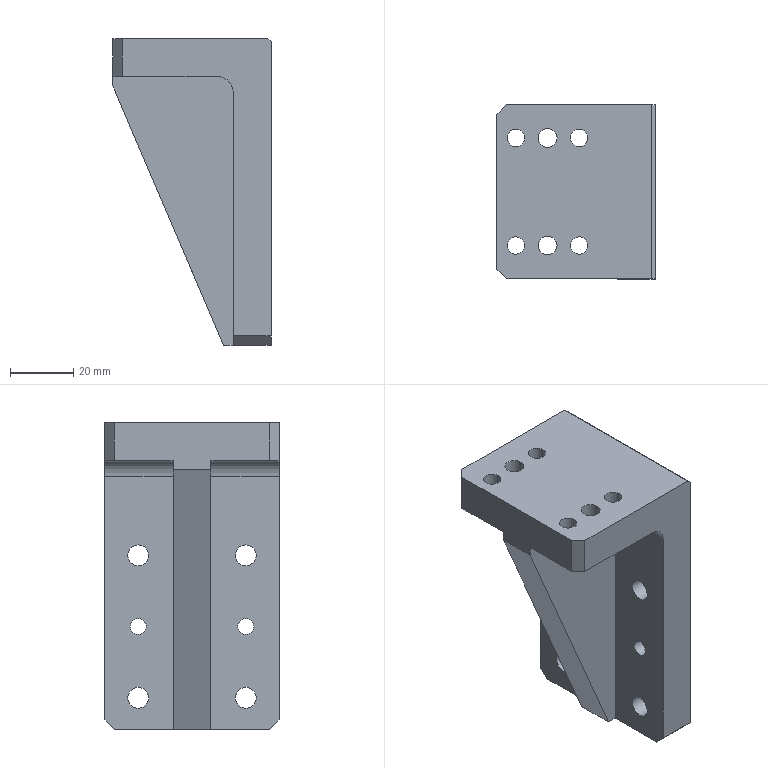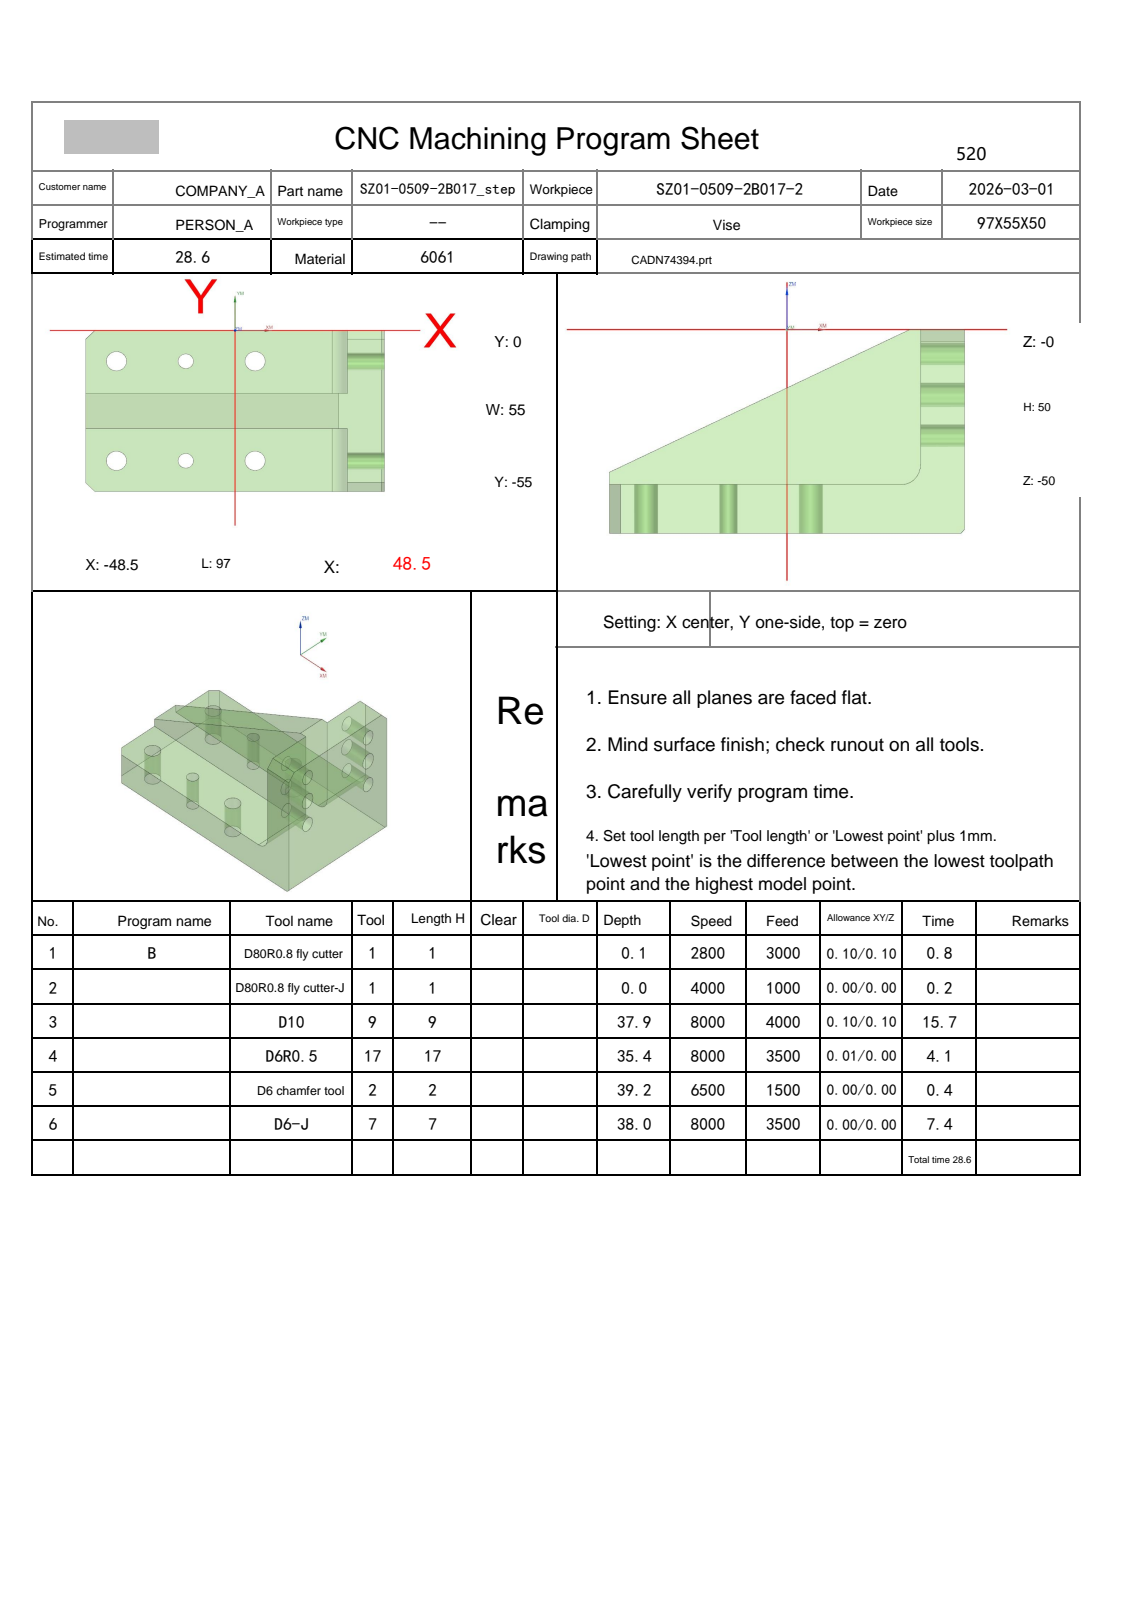NC program | NX | posted by the shop | part box 50 x 55 x 97 mm
Lines 8313 to 10086 of 18128:
N4 T17 M06
(D6R0.5  D=6. R=0.5 H=17 ce=0.01 di=0.00)
G00 G90 G54 X30.202 Y-.343 M03 S8000
G43 H17 Z14.5
M08
Z.429
G01 Z-.071 F3500.
X35.426 Y-.215
X35.55 Y-.212
X49.574
Y-.177 Z-.106
Y-.142 Z-.141
X35.55 Y-.141
X35.426 Y-.144
Y-.106 Z-.177
Y-.074 Z-.212
X35.55 Y-.071
X48.5
X49.574
Y-.035 Z-.247
X49.575 Y0.0 Z-.283
X48.5
X35.55
X35.425 Y-.003
Y.035 Z-.318
Y.068 Z-.354
X35.55 Y.071
X48.5
X49.575
Y.106 Z-.389
Y.141 Z-.424
X48.5
X35.55
X35.425 Y.138
X35.424 Y.177 Z-.46
Y.209 Z-.495
X35.55 Y.212
X48.5
X49.576
Y.247 Z-.53
Y.283 Z-.566
X48.5
X35.55
X35.424 Y.28
Y.318 Z-.601
X35.423 Y.35 Z-.636
X35.55 Y.354
X48.5
X49.577 Y.353
Y.389 Z-.672
Y.424 Z-.707
X48.5
X35.55
X35.423 Y.421
Y.46 Z-.742
Y.492 Z-.778
X35.55 Y.495
X48.5
X49.577
X49.578 Y.53 Z-.813
Y.566 Z-.849
X48.5
X35.55
X35.422 Y.563
Y.601 Z-.884
Y.633 Z-.919
X35.55 Y.636
X48.5
X49.578
Y.672 Z-.955
Y.707 Z-.99
X48.5
X35.55
X35.422 Y.704
X35.421 Y.742 Z-1.025
Y.775 Z-1.061
X35.55 Y.778
X48.5
X49.579
Y.813 Z-1.096
Y.848 Z-1.131
X48.5
X35.55
X35.421 Y.845
Y.884 Z-1.167
Y.916 Z-1.202
X35.55 Y.919
X48.5
X49.579
Y.955 Z-1.237
Y.99 Z-1.273
X48.5
X35.55
X35.421 Y.987
Y1.025 Z-1.308
Y1.058 Z-1.344
X35.55 Y1.061
X48.5
X49.579 Y1.06
Y1.096 Z-1.379
Y1.131 Z-1.414
X48.5
X36.5
X35.421
Y1.167 Z-1.45
Y1.199 Z-1.485
X35.55 Y1.202
X48.5
X49.579
Y1.237 Z-1.52
Y1.273 Z-1.556
X48.5
X35.55
X35.421 Y1.27
Y1.308 Z-1.591
Y1.34 Z-1.626
X35.55 Y1.343
X48.5
X49.579
Y1.379 Z-1.662
Y1.414 Z-1.697
X48.5
X35.55
X35.421 Y1.411
Y1.45 Z-1.732
Y1.482 Z-1.768
X35.55 Y1.485
X48.5
X49.579
Y1.52 Z-1.803
Y1.555 Z-1.838
X48.5 Y1.556
X35.55
X35.421 Y1.553
Y1.591 Z-1.874
Y1.623 Z-1.909
X35.55 Y1.626
X48.5
X49.579
Y1.662 Z-1.945
Y1.697 Z-1.98
X48.5
X35.55
X35.421 Y1.694
Y1.732 Z-2.015
Y1.765 Z-2.051
X35.55 Y1.768
X48.5
X49.579
Y1.803 Z-2.086
Y1.838 Z-2.121
X48.5
X35.55
X35.421 Y1.835
Y1.874 Z-2.157
Y1.906 Z-2.192
X35.55 Y1.909
X48.5
X49.579
Y1.944 Z-2.227
Y1.98 Z-2.263
X48.5
X35.55
X35.421 Y1.977
X35.422 Y2.015 Z-2.298
Y2.048 Z-2.333
X35.55 Y2.051
X48.5
X49.578 Y2.05
Y2.086 Z-2.369
Y2.121 Z-2.404
X48.5
X35.55
X35.422 Y2.118
Y2.157 Z-2.44
Y2.189 Z-2.475
X35.55 Y2.192
X48.5
X49.578
X49.577 Y2.227 Z-2.51
Y2.263 Z-2.546
X48.5
X35.55
X35.423 Y2.26
Y2.298 Z-2.581
Y2.33 Z-2.616
X35.55 Y2.333
X48.5
X49.577
Y2.369 Z-2.652
X49.576 Y2.404 Z-2.687
X48.5
X35.55
X35.424 Y2.401
Y2.439 Z-2.722
Y2.472 Z-2.758
X35.55 Y2.475
X48.5
X49.576
Y2.505 Z-2.788
Y2.535 Z-2.818
X48.5
X35.55
X35.424 Y2.532
X35.425 Y2.566 Z-2.849
Y2.593 Z-2.879
X35.55 Y2.596
X48.5
X49.575
Y2.626 Z-2.909
Y2.656 Z-2.939
X48.5 Y2.657
X35.55
X35.425 Y2.654
Y2.687 Z-2.97
Y2.714 Z-3.
X35.55 Y2.717
X48.5
X49.575
G00 Z14.5
X54.722 Y-54.788
Z.429
G01 Z-.071
X49.574
X35.552
X35.427 Y-54.785
X35.426 Y-54.823 Z-.106
Y-54.856 Z-.141
X35.552 Y-54.859
X49.574 Y-54.858
Y-54.894 Z-.177
Y-54.929 Z-.212
X48.5
X35.552
X35.426 Y-54.926
X35.425 Y-54.965 Z-.247
Y-54.997 Z-.283
X35.552 Y-55.
X48.5
X49.575
Y-55.035 Z-.318
Y-55.071 Z-.354
X48.5
X35.552
X35.425 Y-55.068
Y-55.106 Z-.389
Y-55.138 Z-.424
X35.552 Y-55.141
X48.5
X49.575
X49.576 Y-55.177 Z-.46
Y-55.212 Z-.495
X48.5
X35.552
X35.424 Y-55.209
Y-55.247 Z-.53
Y-55.28 Z-.566
X35.552 Y-55.283
X48.5
X49.576
Y-55.318 Z-.601
X49.577 Y-55.353 Z-.636
X48.5 Y-55.354
X35.552
X35.423 Y-55.35
Y-55.389 Z-.672
Y-55.421 Z-.707
X35.552 Y-55.424
X48.5
X49.577
Y-55.46 Z-.742
Y-55.495 Z-.778
X48.5
X35.552
X35.423 Y-55.492
Y-55.53 Z-.813
X35.422 Y-55.563 Z-.849
X35.552 Y-55.566
X48.5
X49.578 Y-55.565
Y-55.601 Z-.884
Y-55.636 Z-.919
X48.5
X35.552
X35.422 Y-55.633
Y-55.672 Z-.955
Y-55.704 Z-.99
X35.552 Y-55.707
X48.5
X49.579
Y-55.742 Z-1.025
Y-55.778 Z-1.061
X48.5
X35.552
X35.421 Y-55.775
Y-55.813 Z-1.096
Y-55.845 Z-1.131
X35.552 Y-55.848
X48.5
X49.579
Y-55.884 Z-1.167
Y-55.919 Z-1.202
X48.5
X35.552
X35.421 Y-55.916
Y-55.955 Z-1.237
Y-55.987 Z-1.273
X35.552 Y-55.99
X48.5
X49.579
Y-56.025 Z-1.308
Y-56.06 Z-1.344
X48.5 Y-56.061
X35.552
X35.421 Y-56.058
Y-56.096 Z-1.379
Y-56.131 Z-1.414
X36.5
X48.5
X49.579
Y-56.167 Z-1.45
Y-56.202 Z-1.485
X48.5
X35.552
X35.421 Y-56.199
Y-56.237 Z-1.52
Y-56.27 Z-1.556
X35.552 Y-56.273
X48.5
X49.579
Y-56.308 Z-1.591
Y-56.343 Z-1.626
X48.5
X35.552
X35.421 Y-56.34
Y-56.379 Z-1.662
Y-56.411 Z-1.697
X35.552 Y-56.414
X48.5
X49.579
Y-56.45 Z-1.732
Y-56.485 Z-1.768
X48.5
X35.552
X35.421 Y-56.482
Y-56.52 Z-1.803
Y-56.553 Z-1.838
X35.552 Y-56.556
X48.5
X49.579 Y-56.555
Y-56.591 Z-1.874
Y-56.626 Z-1.909
X48.5
X35.552
X35.421 Y-56.623
Y-56.662 Z-1.945
Y-56.694 Z-1.98
X35.552 Y-56.697
X48.5
X49.579
Y-56.732 Z-2.015
Y-56.768 Z-2.051
X48.5
X35.552
X35.421 Y-56.765
Y-56.803 Z-2.086
Y-56.835 Z-2.121
X35.552 Y-56.838
X48.5
X49.579
Y-56.874 Z-2.157
Y-56.909 Z-2.192
X48.5
X35.552
X35.421 Y-56.906
Y-56.944 Z-2.227
Y-56.977 Z-2.263
X35.552 Y-56.98
X48.5
X49.579
X49.578 Y-57.015 Z-2.298
Y-57.05 Z-2.333
X48.5 Y-57.051
X35.552
X35.422 Y-57.048
Y-57.086 Z-2.369
Y-57.118 Z-2.404
X35.552 Y-57.121
X48.5
X49.578
Y-57.157 Z-2.44
X49.577 Y-57.192 Z-2.475
X48.5
X35.552
X35.422 Y-57.189
X35.423 Y-57.227 Z-2.51
Y-57.26 Z-2.546
X35.552 Y-57.263
X48.5
X49.577
Y-57.298 Z-2.581
Y-57.333 Z-2.616
X48.5
X35.552
X35.423 Y-57.33
Y-57.369 Z-2.652
X35.424 Y-57.401 Z-2.687
X35.552 Y-57.404
X48.5
X49.576
Y-57.439 Z-2.722
Y-57.475 Z-2.758
X48.5
X35.552
X35.424 Y-57.472
Y-57.505 Z-2.788
Y-57.532 Z-2.818
X35.552 Y-57.535
X48.5
X49.576
Y-57.566 Z-2.849
X49.575 Y-57.596 Z-2.879
X48.5
X35.552
X35.425 Y-57.593
Y-57.626 Z-2.909
Y-57.654 Z-2.939
X35.552 Y-57.657
X48.5
X49.575 Y-57.656
Y-57.687 Z-2.97
Y-57.717 Z-3.
X48.5
X35.552
X35.425 Y-57.714
G00 Z14.5
G00 G90 X27.799 Y-34.576 M03 S8000
Z14.5
Z.461
G01 Z-.039 F3500.
X30.799
Y-20.424
X30.75 Z-.059
X30.707 Z-.079
X30.704 Y-21.5
Y-33.5
X30.707 Y-34.576
X30.658 Y-34.577 Z-.098
X30.615 Z-.118
X30.612 Y-33.5
Y-21.5
X30.615 Y-20.423
X30.566 Z-.137
X30.523 Z-.157
X30.52 Y-21.5
Y-33.5
X30.523 Y-34.577
X30.474 Y-34.578 Z-.177
X30.431 Z-.196
X30.428 Y-33.5
Y-21.5
X30.431 Y-20.422
X30.382 Z-.216
X30.339 Y-20.421 Z-.236
X30.336 Y-21.5
Y-33.5
X30.339 Y-34.578
X30.29 Y-34.579 Z-.255
X30.247 Z-.275
X30.244 Y-33.5
Y-21.5
X30.247 Y-20.421
X30.198 Z-.294
X30.155 Y-20.42 Z-.314
X30.152 Y-21.5
Y-33.5
X30.155 Y-34.58
X30.106 Z-.334
X30.063 Z-.353
X30.06 Y-33.5
Y-21.5
X30.063 Y-20.42
X30.014 Y-20.419 Z-.373
X29.971 Z-.393
X29.968 Y-21.5
Y-33.5
X29.971 Y-34.581
X29.922 Z-.412
X29.879 Z-.432
X29.876 Y-33.5
Y-21.5
X29.879 Y-20.419
X29.83 Y-20.418 Z-.451
X29.787 Z-.471
X29.784 Y-21.5
Y-33.5
X29.787 Y-34.582
X29.738 Z-.491
X29.695 Y-34.583 Z-.51
X29.692 Y-33.5
Y-21.5
X29.695 Y-20.418
X29.646 Y-20.417 Z-.53
X29.603 Z-.55
X29.6 Y-21.5
Y-33.5
X29.603 Y-34.583
X29.554 Z-.569
X29.511 Y-34.584 Z-.589
X29.508 Y-33.5
Y-21.5
X29.511 Y-20.416
X29.462 Z-.608
X29.419 Z-.628
X29.416 Y-21.5
Y-33.5
X29.419 Y-34.584
X29.37 Y-34.585 Z-.648
X29.327 Z-.667
X29.324 Y-33.5
Y-21.5
X29.327 Y-20.415
X29.278 Z-.687
X29.235 Z-.707
X29.232 Y-21.5
Y-33.5
X29.235 Y-34.585
X29.186 Y-34.586 Z-.726
X29.143 Z-.746
X29.14 Y-33.5
Y-21.5
X29.143 Y-20.414
X29.094 Z-.766
X29.051 Z-.785
X29.048 Y-21.5
Y-33.5
X29.051 Y-34.586
X29.002 Y-34.587 Z-.805
X28.959 Z-.824
X28.956 Y-33.5
Y-21.5
X28.959 Y-20.413
X28.91 Z-.844
X28.867 Z-.864
X28.864 Y-21.5
Y-33.5
X28.867 Y-34.587
X28.818 Y-34.588 Z-.883
X28.775 Z-.903
X28.772 Y-33.5
Y-21.5
X28.775 Y-20.412
X28.726 Z-.923
X28.683 Z-.942
X28.68 Y-21.5
Y-33.5
X28.683 Y-34.588
X28.634 Z-.962
X28.591 Y-34.589 Z-.981
X28.588 Y-33.5
Y-21.5
X28.591 Y-20.411
X28.542 Z-1.001
X28.499 Z-1.021
X28.496 Y-21.5
Y-33.5
X28.499 Y-34.589
X28.45 Z-1.04
X28.407 Y-34.59 Z-1.06
X28.405 Y-33.5
Y-21.5
X28.407 Y-20.411
X28.359 Y-20.41 Z-1.08
X28.315 Z-1.099
X28.313 Y-21.5
Y-33.5
X28.315 Y-34.59
X28.267 Z-1.119
X28.223 Z-1.138
X28.221 Y-33.5
Y-21.5
X28.223 Y-20.41
X28.175 Z-1.158
X28.131 Y-20.409 Z-1.178
X28.129 Y-21.5
Y-33.5
X28.131 Y-34.591
X28.083 Z-1.197
X28.039 Z-1.217
X28.037 Y-33.5
Y-21.5
X28.039 Y-20.409
X27.991 Z-1.237
X27.947 Z-1.256
X27.945 Y-21.5
Y-33.5
X27.947 Y-34.591
X27.899 Y-34.592 Z-1.276
X27.855 Z-1.295
X27.853 Y-33.5
Y-21.5
X27.855 Y-20.408
X27.807 Z-1.315
X27.763 Z-1.335
X27.761 Y-21.5
Y-33.5
X27.763 Y-34.592
X27.715 Z-1.354
X27.671 Y-34.593 Z-1.374
X27.669 Y-33.5
Y-21.5
X27.671 Y-20.407
X27.623 Z-1.394
X27.579 Z-1.413
X27.577 Y-21.5
Y-33.5
X27.579 Y-34.593
X27.531 Z-1.433
X27.487 Z-1.452
X27.485 Y-33.5
Y-21.5
X27.487 Y-20.407
X27.439 Y-20.406 Z-1.472
X27.395 Z-1.492
X27.393 Y-21.5
Y-33.5
X27.395 Y-34.594
X27.347 Z-1.511
X27.303 Z-1.531
X27.301 Y-33.5
Y-21.5
X27.303 Y-20.406
X27.255 Z-1.551
X27.211 Z-1.57
X27.209 Y-21.5
Y-33.5
X27.211 Y-34.594
X27.163 Y-34.595 Z-1.59
X27.119 Z-1.61
X27.117 Y-33.5
Y-21.5
X27.119 Y-20.405
X27.071 Z-1.629
X27.027 Z-1.649
X27.025 Y-21.5
Y-33.5
X27.027 Y-34.595
X26.979 Z-1.668
X26.935 Z-1.688
X26.933 Y-33.5
Y-21.5
X26.935 Y-20.405
X26.887 Z-1.708
X26.843 Z-1.727
X26.841 Y-21.5
Y-33.5
X26.843 Y-34.595
X26.795 Y-34.596 Z-1.747
X26.751 Z-1.767
X26.749 Y-33.5
Y-21.5
X26.751 Y-20.404
X26.703 Z-1.786
X26.659 Z-1.806
X26.657 Y-21.5
Y-33.5
X26.659 Y-34.596
X26.611 Z-1.825
X26.567 Z-1.845
X26.565 Y-33.5
Y-21.5
X26.567 Y-20.404
X26.519 Z-1.865
X26.475 Z-1.884
X26.473 Y-21.5
Y-33.5
X26.475 Y-34.596
X26.427 Z-1.904
X26.383 Z-1.924
X26.381 Y-33.5
Y-21.5
X26.383 Y-20.404
X26.335 Z-1.943
X26.292 Y-20.403 Z-1.963
X26.289 Y-21.5
Y-33.5
X26.292 Y-34.597
X26.243 Z-1.982
X26.2 Z-2.002
X26.197 Y-33.5
Y-21.5
X26.2 Y-20.403
X26.151 Z-2.022
X26.108 Z-2.041
X26.105 Y-21.5
Y-33.5
X26.108 Y-34.597
X26.059 Z-2.061
X26.016 Z-2.081
X26.013 Y-33.5
Y-21.5
X26.016 Y-20.403
X25.967 Z-2.1
X25.924 Z-2.12
X25.921 Y-21.5
Y-33.5
X25.924 Y-34.597
X25.875 Z-2.139
X25.832 Z-2.159
X25.829 Y-33.5
Y-21.5
X25.832 Y-20.403
X25.783 Z-2.179
X25.74 Y-20.402 Z-2.198
X25.737 Y-21.5
Y-33.5
X25.74 Y-34.598
X25.691 Z-2.218
X25.648 Z-2.238
X25.645 Y-33.5
Y-21.5
X25.648 Y-20.402
X25.599 Z-2.257
X25.556 Z-2.277
X25.553 Y-21.5
Y-33.5
X25.556 Y-34.598
X25.507 Z-2.297
X25.464 Z-2.316
X25.461 Y-33.5
Y-21.5
X25.464 Y-20.402
X25.415 Z-2.336
X25.372 Z-2.355
X25.369 Y-21.5
Y-33.5
X25.372 Y-34.598
X25.323 Z-2.375
X25.28 Z-2.395
X25.277 Y-33.5
Y-21.5
X25.28 Y-20.402
X25.231 Z-2.414
X25.188 Z-2.434
X25.185 Y-21.5
Y-33.5
X25.188 Y-34.598
X25.139 Z-2.454
X25.096 Z-2.473
X25.093 Y-33.5
Y-21.5
X25.096 Y-20.401
X25.048 Z-2.493
X25.004 Z-2.512
X25.002 Y-21.5
Y-33.5
X25.004 Y-34.598
X24.956 Z-2.532
X24.912 Y-34.599 Z-2.552
X24.91 Y-33.5
Y-21.5
X24.912 Y-20.401
X24.864 Z-2.571
X24.82 Z-2.591
X24.818 Y-21.5
Y-33.5
X24.82 Y-34.599
X24.772 Z-2.611
X24.728 Z-2.63
X24.726 Y-33.5
Y-21.5
X24.728 Y-20.401
X24.68 Z-2.65
X24.636 Z-2.669
X24.634 Y-21.5
Y-33.5
X24.636 Y-34.599
X24.588 Z-2.689
X24.544 Z-2.709
X24.542 Y-33.5
Y-21.5
X24.544 Y-20.401
X24.496 Z-2.728
X24.452 Z-2.748
X24.45 Y-21.5
Y-33.5
X24.452 Y-34.599
X24.404 Z-2.768
X24.36 Z-2.787
X24.358 Y-33.5
Y-21.5
X24.36 Y-20.401
X24.312 Z-2.807
X24.268 Z-2.826
X24.266 Y-21.5
Y-33.5
X24.268 Y-34.599
X24.22 Z-2.846
X24.176 Z-2.866
X24.174 Y-33.5
Y-21.5
X24.176 Y-20.401
X24.128 Z-2.885
X24.084 Z-2.905
X24.082 Y-21.5
Y-33.5
X24.084 Y-34.599
X24.036 Z-2.925
X23.992 Z-2.944
X23.99 Y-33.5
Y-21.5
X23.992 Y-20.401
X23.944 Z-2.964
X23.9 Z-2.983
X23.898 Y-21.5
Y-33.5
X23.9 Y-34.599
X23.852 Z-3.003
X23.808 Z-3.023
X23.806 Y-33.5
Y-21.5
X23.808 Y-20.401
X23.76 Z-3.042
X23.716 Z-3.062
X23.714 Y-21.5
Y-33.5
X23.716 Y-34.599
X23.668 Z-3.082
X23.624 Z-3.101
X23.622 Y-33.5
Y-21.5
X23.624 Y-20.401
X23.576 Z-3.121
X23.532 Z-3.141
X23.53 Y-21.5
Y-33.5
X23.532 Y-34.599
X23.484 Z-3.16
X23.44 Z-3.18
X23.438 Y-33.5
Y-21.5
X23.44 Y-20.401
X23.392 Z-3.199
X23.348 Y-20.4 Z-3.219
X23.346 Y-21.5
Y-33.5
X23.348 Y-34.599
X23.3 Z-3.239
X23.256 Z-3.258
X23.254 Y-33.5
Y-21.5
X23.256 Y-20.4
X23.208 Z-3.278
X23.164 Z-3.298
X23.162 Y-21.5
Y-33.5
X23.164 Y-34.599
X23.116 Y-34.6 Z-3.317
X23.072 Z-3.337
X23.07 Y-33.5
Y-21.5
X23.072 Y-20.4
X23.024 Z-3.356
X22.98 Z-3.376
X22.978 Y-21.5
Y-33.5
X22.98 Y-34.6
X22.932 Z-3.396
X22.888 Z-3.415
X22.886 Y-33.5
Y-21.5
X22.888 Y-20.4
X22.84 Z-3.435
X22.797 Z-3.455
X22.794 Y-21.5
Y-33.5
X22.797 Y-34.6
X22.748 Z-3.474
X22.705 Z-3.494
X22.702 Y-33.5
Y-21.5
X22.705 Y-20.4
X22.656 Z-3.513
X22.613 Z-3.533
X22.61 Y-21.5
Y-33.5
X22.613 Y-34.6
X22.564 Z-3.553
X22.521 Z-3.572
X22.518 Y-33.5
Y-21.5
X22.521 Y-20.4
X22.472 Z-3.592
X22.429 Z-3.612
X22.426 Y-21.5
Y-33.5
X22.429 Y-34.6
X22.38 Z-3.631
X22.337 Z-3.651
X22.334 Y-33.5
Y-21.5
X22.337 Y-20.4
X22.288 Z-3.67
X22.245 Z-3.69
X22.242 Y-21.5
Y-33.5
X22.245 Y-34.6
X22.196 Z-3.71
X22.153 Z-3.729
X22.15 Y-33.5
Y-21.5
X22.153 Y-20.4
X22.104 Z-3.749
X22.061 Z-3.769
X22.058 Y-21.5
Y-33.5
X22.061 Y-34.6
X22.012 Z-3.788
X21.969 Z-3.808
X21.966 Y-33.5
Y-21.5
X21.969 Y-20.4
X21.92 Z-3.828
X21.877 Z-3.847
X21.874 Y-21.5
Y-33.5
X21.877 Y-34.6
X21.828 Z-3.867
X21.785 Z-3.886
X21.782 Y-33.5
Y-21.5
X21.785 Y-20.4
X21.736 Z-3.906
X21.693 Z-3.926
X21.691 Y-21.5
Y-33.5
X21.693 Y-34.6
X21.645 Z-3.945
X21.601 Z-3.965
X21.599 Y-33.5
Y-21.5
X21.601 Y-20.4
X21.553 Z-3.985
X21.509 Z-4.004
X21.507 Y-21.5
Y-33.5
X21.509 Y-34.6
X21.461 Z-4.024
X21.417 Z-4.043
X21.415 Y-33.5
Y-21.5
X21.417 Y-20.4
X21.369 Z-4.063
X21.325 Z-4.083
X21.323 Y-21.5
Y-33.5
X21.325 Y-34.6
X21.277 Z-4.102
X21.233 Z-4.122
X21.231 Y-33.5
Y-21.5
X21.233 Y-20.4
X21.185 Z-4.142
X21.141 Z-4.161
X21.139 Y-21.5
Y-33.5
X21.141 Y-34.6
X21.093 Z-4.181
X21.049 Z-4.2
X21.047 Y-33.5
Y-21.5
X21.049 Y-20.4
X21.001 Z-4.22
X20.957 Z-4.24
X20.955 Y-21.5
Y-33.5
X20.957 Y-34.6
X20.909 Z-4.259
X20.865 Z-4.279
X20.863 Y-33.5
Y-21.5
X20.865 Y-20.4
X20.817 Z-4.299
X20.773 Z-4.318
X20.771 Y-21.5
Y-33.5
X20.773 Y-34.6
X20.725 Z-4.338
X20.681 Z-4.357
X20.679 Y-33.5
Y-21.5
X20.681 Y-20.4
X20.633 Z-4.377
X20.589 Z-4.397
X20.587 Y-21.5
Y-33.5
X20.589 Y-34.6
X20.541 Z-4.416
X20.497 Z-4.436
X20.495 Y-33.5
Y-21.5
X20.497 Y-20.4
X20.449 Z-4.456
X20.405 Z-4.475
X20.403 Y-21.5
Y-33.5
X20.405 Y-34.6
X20.357 Z-4.495
X20.313 Z-4.515
X20.311 Y-33.5
Y-21.5
X20.313 Y-20.4
X20.265 Z-4.534
X20.221 Z-4.554
X20.219 Y-21.5
Y-33.5
X20.221 Y-34.6
X20.173 Z-4.573
X20.129 Z-4.593
X20.127 Y-33.5
Y-21.5
X20.129 Y-20.4
X20.081 Z-4.613
X20.037 Z-4.632
X20.035 Y-21.5
Y-33.5
X20.037 Y-34.6
X19.989 Z-4.652
X19.945 Z-4.672
X19.943 Y-33.5
Y-21.5
X19.945 Y-20.4
X19.897 Z-4.691
X19.853 Z-4.711
X19.851 Y-21.5
Y-33.5
X19.853 Y-34.6
X19.805 Z-4.73
X19.761 Z-4.75
X19.759 Y-33.5
Y-21.5
X19.761 Y-20.4
X19.713 Z-4.77
X19.669 Z-4.789
X19.667 Y-21.5
Y-33.5
X19.669 Y-34.6
X19.621 Z-4.809
X19.577 Z-4.829
X19.575 Y-33.5
Y-21.5
X19.577 Y-20.4
X19.529 Z-4.848
X19.485 Z-4.868
X19.483 Y-21.5
Y-33.5
X19.485 Y-34.6
X19.437 Z-4.887
X19.394 Z-4.907
X19.391 Y-33.5
Y-21.5
X19.394 Y-20.4
X19.345 Z-4.927
X19.302 Z-4.946
X19.299 Y-21.5
Y-33.5
X19.302 Y-34.6
X19.253 Z-4.966
X19.21 Z-4.986
X19.207 Y-33.5
Y-21.5
X19.21 Y-20.4
X19.161 Z-5.005
X19.118 Z-5.025
X19.115 Y-21.5
Y-33.5
X19.118 Y-34.6
X19.069 Z-5.044
X19.026 Z-5.064
X19.023 Y-33.5
Y-21.5
X19.026 Y-20.4
X18.977 Z-5.084
X18.934 Z-5.103
X18.931 Y-21.5
Y-33.5
X18.934 Y-34.6
X18.885 Z-5.123
X18.842 Z-5.143
X18.839 Y-33.5
Y-21.5
X18.842 Y-20.4
X18.793 Z-5.162
X18.75 Z-5.182
X18.747 Y-21.5
Y-33.5
X18.75 Y-34.6
X18.701 Z-5.201
X18.658 Z-5.221
X18.655 Y-33.5
Y-21.5
X18.658 Y-20.4
X18.609 Z-5.241
X18.566 Z-5.26
X18.563 Y-21.5
Y-33.5
X18.566 Y-34.6
X18.517 Z-5.28
X18.474 Z-5.3
X18.471 Y-33.5
Y-21.5
X18.474 Y-20.4
X18.425 Z-5.319
X18.382 Z-5.339
X18.38 Y-21.5
Y-33.5
X18.382 Y-34.6
X18.334 Z-5.359
X18.29 Z-5.378
X18.288 Y-33.5
Y-21.5
X18.29 Y-20.4
X18.242 Z-5.398
X18.198 Z-5.417
X18.196 Y-21.5
Y-33.5
X18.198 Y-34.6
X18.15 Z-5.437
X18.106 Z-5.457
X18.104 Y-33.5
Y-21.5
X18.106 Y-20.4
X18.058 Z-5.476
X18.014 Z-5.496
X18.012 Y-21.5
Y-33.5
X18.014 Y-34.6
X17.966 Z-5.516
X17.922 Z-5.535
X17.92 Y-33.5
Y-21.5
X17.922 Y-20.4
X17.874 Z-5.555
X17.83 Z-5.574
X17.828 Y-21.5
Y-33.5
X17.83 Y-34.6
X17.782 Z-5.594
X17.738 Z-5.614
X17.736 Y-33.5
Y-21.5
X17.738 Y-20.4
X17.69 Z-5.633
X17.646 Z-5.653
X17.644 Y-21.5
Y-33.5
X17.646 Y-34.6
X17.598 Z-5.673
X17.554 Z-5.692
X17.552 Y-33.5
Y-21.5
X17.554 Y-20.4
X17.506 Z-5.712
X17.462 Z-5.731
X17.46 Y-21.5
Y-33.5
X17.462 Y-34.6
X17.414 Z-5.751
X17.37 Z-5.771
X17.368 Y-33.5
Y-21.5
X17.37 Y-20.4
X17.322 Z-5.79
X17.278 Z-5.81
X17.276 Y-21.5
Y-33.5
X17.278 Y-34.6
X17.23 Z-5.83
X17.186 Z-5.849
X17.184 Y-33.5
Y-21.5
X17.186 Y-20.4
X17.138 Z-5.869
X17.094 Z-5.888
X17.092 Y-21.5
Y-33.5
X17.094 Y-34.6
X17.046 Z-5.908
X17.002 Z-5.928
X17. Y-33.5
Y-21.5
X17.002 Y-20.4
X16.954 Z-5.947
X16.91 Z-5.967
X16.908 Y-21.5
Y-33.5
X16.91 Y-34.6
X16.862 Z-5.987
X16.818 Z-6.006
X16.816 Y-33.5
Y-21.5
X16.818 Y-20.4
X16.77 Z-6.026
X16.726 Z-6.046
X16.724 Y-21.5
Y-33.5
X16.726 Y-34.6
X16.678 Z-6.065
X16.634 Z-6.085
X16.632 Y-33.5
Y-21.5
X16.634 Y-20.4
X16.586 Z-6.104
X16.542 Z-6.124
X16.54 Y-21.5
Y-33.5
X16.542 Y-34.6
X16.494 Z-6.144
X16.45 Z-6.163
X16.448 Y-33.5
Y-21.5
X16.45 Y-20.4
X16.402 Z-6.183
X16.358 Z-6.203
X16.356 Y-21.5
Y-33.5
X16.358 Y-34.6
X16.31 Z-6.222
X16.266 Z-6.242
X16.264 Y-33.5
Y-21.5
X16.266 Y-20.4
X16.218 Z-6.261
X16.174 Z-6.281
X16.172 Y-21.5
Y-33.5
X16.174 Y-34.6
X16.126 Z-6.301
X16.083 Z-6.32
X16.08 Y-33.5
Y-21.5
X16.083 Y-20.4
X16.034 Z-6.34
X15.99 Z-6.36
X15.988 Y-21.5
Y-33.5
X15.99 Y-34.6
X15.942 Z-6.379
X15.899 Z-6.399
X15.896 Y-33.5
Y-21.5
X15.899 Y-20.4
X15.85 Z-6.418
X15.807 Z-6.438
X15.804 Y-21.5
Y-33.5
X15.807 Y-34.6
X15.758 Z-6.458
X15.715 Z-6.477
X15.712 Y-33.5
Y-21.5
X15.715 Y-20.4
X15.666 Z-6.497
X15.623 Z-6.517
X15.62 Y-21.5
Y-33.5
X15.623 Y-34.6
X15.574 Z-6.536
X15.531 Z-6.556
X15.528 Y-33.5
Y-21.5
X15.531 Y-20.4
X15.482 Z-6.575
X15.439 Z-6.595
X15.436 Y-21.5
Y-33.5
X15.439 Y-34.6
X15.39 Z-6.615
X15.347 Z-6.634
X15.344 Y-33.5
Y-21.5
X15.347 Y-20.4
X15.298 Z-6.654
X15.255 Z-6.674
X15.252 Y-21.5
Y-33.5
X15.255 Y-34.6
X15.206 Z-6.693
X15.163 Z-6.713
X15.16 Y-33.5
Y-21.5
X15.163 Y-20.4
X15.114 Z-6.732
X15.071 Z-6.752
X15.068 Y-21.5
Y-33.5
X15.071 Y-34.6
X15.023 Z-6.772
X14.979 Z-6.791
X14.977 Y-33.5
Y-21.5
X14.979 Y-20.4
X14.931 Z-6.811
X14.887 Z-6.831
X14.885 Y-21.5
Y-33.5
X14.887 Y-34.6
X14.839 Z-6.85
X14.795 Z-6.87
X14.793 Y-33.5
Y-21.5
X14.795 Y-20.4
X14.747 Z-6.89
X14.703 Z-6.909
X14.701 Y-21.5
Y-33.5
X14.703 Y-34.6
X14.655 Z-6.929
X14.611 Z-6.948
X14.609 Y-33.5
Y-21.5
X14.611 Y-20.4
X14.563 Z-6.968
X14.519 Z-6.988
X14.517 Y-21.5
Y-33.5
X14.519 Y-34.6
X14.471 Z-7.007
X14.427 Z-7.027
X14.425 Y-33.5
Y-21.5
X14.427 Y-20.4
X14.379 Z-7.047
X14.335 Z-7.066
X14.333 Y-21.5
Y-33.5
X14.335 Y-34.6
X14.287 Z-7.086
X14.243 Z-7.105
X14.241 Y-33.5
Y-21.5
X14.243 Y-20.4
X14.195 Z-7.125
X14.151 Z-7.145
X14.149 Y-21.5
Y-33.5
X14.151 Y-34.6
X14.103 Z-7.164
X14.059 Z-7.184
X14.057 Y-33.5
Y-21.5
X14.059 Y-20.4
X14.011 Z-7.204
X13.967 Z-7.223
X13.965 Y-21.5
Y-33.5
X13.967 Y-34.6
X13.919 Z-7.243
X13.875 Z-7.262
X13.873 Y-33.5
Y-21.5
X13.875 Y-20.4
X13.827 Z-7.282
X13.783 Z-7.302
X13.781 Y-21.5
Y-33.5
X13.783 Y-34.6
X13.735 Z-7.321
X13.691 Z-7.341
X13.689 Y-33.5
Y-21.5
X13.691 Y-20.4
X13.643 Z-7.361
X13.599 Z-7.38
X13.597 Y-21.5
Y-33.5
X13.599 Y-34.6
X13.551 Z-7.4
X13.507 Z-7.419
X13.505 Y-33.5
Y-21.5
X13.507 Y-20.4
X13.459 Z-7.439
X13.415 Z-7.459
X13.413 Y-21.5
Y-33.5
X13.415 Y-34.6
X13.367 Z-7.478
X13.323 Z-7.498
X13.321 Y-33.5
Y-21.5
X13.323 Y-20.4
X13.275 Z-7.518
X13.231 Z-7.537
X13.229 Y-21.5
Y-33.5
X13.231 Y-34.6
X13.183 Z-7.557
X13.139 Z-7.577
X13.137 Y-33.5
Y-21.5
X13.139 Y-20.4
X13.091 Z-7.596
X13.047 Z-7.616
X13.045 Y-21.5
Y-33.5
X13.047 Y-34.6
X12.999 Z-7.635
X12.955 Z-7.655
X12.953 Y-33.5
Y-21.5
X12.955 Y-20.4
X12.907 Z-7.675
X12.863 Z-7.694
X12.861 Y-21.5
Y-33.5
X12.863 Y-34.6
X12.815 Z-7.714
X12.772 Z-7.734
X12.769 Y-33.5
Y-21.5
X12.772 Y-20.4
X12.723 Z-7.753
X12.68 Z-7.773
X12.677 Y-21.5
Y-33.5
X12.68 Y-34.6
X12.631 Z-7.792
X12.588 Z-7.812
X12.585 Y-33.5
Y-21.5
X12.588 Y-20.4
X12.539 Z-7.832
X12.496 Z-7.851
X12.493 Y-21.5
Y-33.5
X12.496 Y-34.6
X12.447 Z-7.871
X12.404 Z-7.891
X12.401 Y-33.5
Y-21.5
X12.404 Y-20.4
X12.355 Z-7.91
X12.312 Z-7.93
X12.309 Y-21.5
Y-33.5
X12.312 Y-34.6
X12.263 Z-7.949
X12.22 Z-7.969
X12.217 Y-33.5
Y-21.5
X12.22 Y-20.4
X12.171 Z-7.989
X12.128 Z-8.008
X12.125 Y-21.5
Y-33.5
X12.128 Y-34.6
X12.079 Z-8.028
X12.036 Z-8.048
X12.033 Y-33.5
Y-21.5
X12.036 Y-20.4
X11.987 Z-8.067
X11.944 Z-8.087
X11.941 Y-21.5
Y-33.5
X11.944 Y-34.6
X11.895 Z-8.106
X11.852 Z-8.126
X11.849 Y-33.5
Y-21.5
X11.852 Y-20.4
X11.803 Z-8.146
X11.76 Z-8.165
X11.757 Y-21.5
Y-33.5
X11.76 Y-34.6
X11.712 Z-8.185
X11.668 Z-8.205
X11.666 Y-33.5
Y-21.5
X11.668 Y-20.4
X11.62 Z-8.224
X11.576 Z-8.244
X11.574 Y-21.5
Y-33.5
X11.576 Y-34.6
X11.528 Z-8.263
X11.482 Z-8.283
Y-33.5
Y-21.5
Y-20.4
X11.436 Z-8.303
X11.392 Z-8.322
X11.39 Y-21.5
Y-33.5
X11.392 Y-34.6
X11.344 Z-8.342
X11.3 Z-8.362
X11.298 Y-33.5
Y-21.5
X11.3 Y-20.4
X11.252 Z-8.381
X11.208 Z-8.401
X11.206 Y-21.5
Y-33.5
X11.208 Y-34.6
X11.16 Z-8.421
X11.116 Z-8.44
X11.114 Y-33.5
Y-21.5
X11.116 Y-20.4
X11.068 Z-8.46
X11.024 Z-8.479
X11.022 Y-21.5
Y-33.5
X11.024 Y-34.6
X10.976 Z-8.499
X10.932 Z-8.519
X10.93 Y-33.5
Y-21.5
X10.932 Y-20.4
X10.884 Z-8.538
X10.84 Z-8.558
X10.838 Y-21.5
Y-33.5
X10.84 Y-34.6
X10.792 Z-8.578
X10.748 Z-8.597
X10.746 Y-33.5
Y-21.5
X10.748 Y-20.4
X10.7 Z-8.617
X10.656 Z-8.636
X10.654 Y-21.5
Y-33.5
X10.656 Y-34.6
X10.608 Z-8.656
X10.564 Z-8.676
X10.562 Y-33.5
Y-21.5
X10.564 Y-20.4
X10.516 Z-8.695
X10.472 Z-8.715
X10.47 Y-21.5
Y-33.5
X10.472 Y-34.6
X10.424 Z-8.735
X10.38 Z-8.754
X10.378 Y-33.5
Y-21.5
X10.38 Y-20.4
X10.332 Z-8.774
X10.288 Z-8.793
X10.286 Y-21.5
Y-33.5
X10.288 Y-34.6
X10.24 Z-8.813
X10.196 Z-8.833
X10.194 Y-33.5
Y-21.5
X10.196 Y-20.4
X10.148 Z-8.852
X10.104 Z-8.872
X10.102 Y-21.5
Y-33.5
X10.104 Y-34.6
X10.056 Z-8.892
X10.012 Z-8.911
X10.01 Y-33.5
Y-21.5
X10.012 Y-20.4
X9.964 Z-8.931
X9.92 Z-8.95
X9.918 Y-21.5
Y-33.5
X9.92 Y-34.6
X9.872 Z-8.97
X9.828 Z-8.99
X9.826 Y-33.5
Y-21.5
X9.828 Y-20.4
X9.78 Z-9.009
X9.736 Z-9.029
X9.734 Y-21.5
Y-33.5
X9.736 Y-34.6
X9.688 Z-9.049
X9.644 Z-9.068
X9.642 Y-33.5
Y-21.5
X9.644 Y-20.4
X9.596 Z-9.088
X9.552 Z-9.108
X9.55 Y-21.5
Y-33.5
X9.552 Y-34.6
X9.504 Z-9.127
X9.46 Z-9.147
X9.458 Y-33.5
Y-21.5
X9.46 Y-20.4
X9.412 Z-9.166
X9.369 Z-9.186
X9.366 Y-21.5
Y-33.5
X9.369 Y-34.6
X9.32 Z-9.206
X9.277 Z-9.225
X9.274 Y-33.5
Y-21.5
X9.277 Y-20.4
X9.228 Z-9.245
X9.185 Z-9.265
X9.182 Y-21.5
Y-33.5
X9.185 Y-34.6
X9.136 Z-9.284
X9.093 Z-9.304
X9.09 Y-33.5
Y-21.5
X9.093 Y-20.4
X9.044 Z-9.323
X9.001 Z-9.343
X8.998 Y-21.5
Y-33.5
X9.001 Y-34.6
X8.952 Z-9.363
X8.909 Z-9.382
X8.906 Y-33.5
Y-21.5
X8.909 Y-20.4
X8.86 Z-9.402
X8.817 Z-9.422
X8.814 Y-21.5
Y-33.5
X8.817 Y-34.6
X8.768 Z-9.441
X8.725 Z-9.461
X8.722 Y-33.5
Y-21.5
X8.725 Y-20.4
X8.676 Z-9.48
X8.633 Z-9.5
X8.63 Y-21.5
Y-33.5
X8.633 Y-34.6
X8.584 Z-9.52
X8.541 Z-9.539
X8.538 Y-33.5
Y-21.5
X8.541 Y-20.4
X8.492 Z-9.559
X8.449 Z-9.579
X8.446 Y-21.5
Y-33.5
X8.449 Y-34.6
X8.4 Z-9.598
X8.357 Z-9.618
X8.355 Y-33.5
Y-21.5
X8.357 Y-20.4
X8.309 Z-9.637
X8.265 Z-9.657
X8.263 Y-21.5
Y-33.5
X8.265 Y-34.6
X8.217 Z-9.677
X8.173 Z-9.696
X8.171 Y-33.5
Y-21.5
X8.173 Y-20.4
X8.125 Z-9.716
X8.081 Z-9.736
X8.079 Y-21.5
Y-33.5
X8.081 Y-34.6
X8.033 Z-9.755
X7.989 Z-9.775
X7.987 Y-33.5
Y-21.5
X7.989 Y-20.4
X7.941 Z-9.795
X7.897 Z-9.814
X7.895 Y-21.5
Y-33.5
X7.897 Y-34.6
X7.849 Z-9.834
X7.805 Z-9.853
X7.803 Y-33.5
Y-21.5
X7.805 Y-20.4
X7.757 Z-9.873
X7.713 Z-9.893
X7.711 Y-21.5
Y-33.5
X7.713 Y-34.6
X7.665 Z-9.912
X7.621 Z-9.932
X7.619 Y-33.5
Y-21.5
X7.621 Y-20.4
X7.573 Z-9.952
X7.529 Z-9.971
X7.527 Y-21.5
Y-33.5
X7.529 Y-34.6
X7.481 Z-9.991
X7.437 Z-10.01
X7.435 Y-33.5
Y-21.5
X7.437 Y-20.4
X7.389 Z-10.03
X7.345 Z-10.05
X7.343 Y-21.5
Y-33.5
X7.345 Y-34.6
X7.297 Z-10.069
X7.253 Z-10.089
X7.251 Y-33.5
Y-21.5
X7.253 Y-20.4
X7.205 Z-10.109
X7.161 Z-10.128
X7.159 Y-21.5
Y-33.5
X7.161 Y-34.6
X7.113 Z-10.148
X7.069 Z-10.167
X7.067 Y-33.5
Y-21.5
X7.069 Y-20.4
X7.021 Z-10.187
X6.977 Z-10.207
X6.975 Y-21.5
Y-33.5
X6.977 Y-34.6
X6.929 Z-10.226
X6.885 Z-10.246
X6.883 Y-33.5
Y-21.5
X6.885 Y-20.4
X6.837 Z-10.266
X6.793 Z-10.285
X6.791 Y-21.5
Y-33.5
X6.793 Y-34.6
X6.745 Z-10.305
X6.701 Z-10.324
X6.699 Y-33.5
Y-21.5
X6.701 Y-20.4
X6.653 Z-10.344
X6.609 Z-10.364
X6.607 Y-21.5
Y-33.5
X6.609 Y-34.6
X6.561 Z-10.383
X6.517 Z-10.403
X6.515 Y-33.5
Y-21.5
X6.517 Y-20.4
X6.469 Z-10.423
X6.425 Z-10.442
X6.423 Y-21.5
Y-33.5
X6.425 Y-34.6
X6.377 Z-10.462
X6.333 Z-10.481
X6.331 Y-33.5
Y-21.5
X6.333 Y-20.4
X6.285 Z-10.501
X6.241 Z-10.521